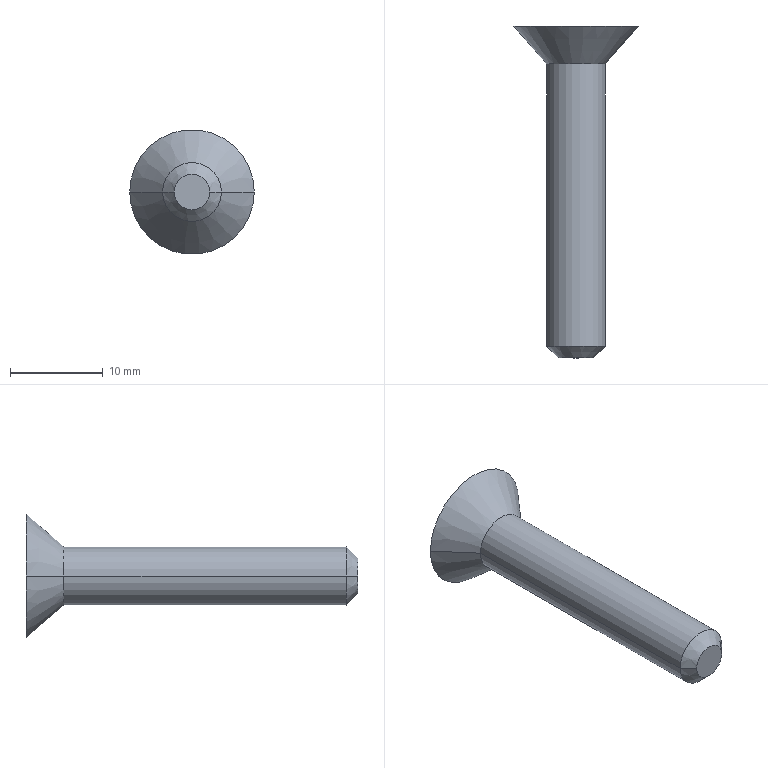Part | NX | features BREP 1 | 1 solid | 15 faces | box 13.46 x 35.839 x 13.46 mm | volume 1303 mm3 | plane 9 | cone 4 | cylinder 2 | commonest cylinder face diameters 6.35 x2
STEP:
#1=CARTESIAN_POINT('',(6.73,0.,0.));
#2=VERTEX_POINT('',#1);
#3=CARTESIAN_POINT('',(3.175,-4.089,0.));
#4=VERTEX_POINT('',#3);
#5=CARTESIAN_POINT('',(3.175,-4.089,0.));
#6=DIRECTION('',(0.6561,0.7547,0.));
#7=VECTOR('',#6,1000.);
#8=LINE('',#5,#7);
#9=EDGE_CURVE('',#2,#4,#8,.F.);
#10=ORIENTED_EDGE('',*,*,#9,.F.);
#11=CARTESIAN_POINT('',(-6.73,0.,0.));
#12=VERTEX_POINT('',#11);
#13=CARTESIAN_POINT('',(0.,0.,0.));
#14=DIRECTION('',(0.,-1.,0.));
#15=DIRECTION('',(1.,0.,0.));
#16=AXIS2_PLACEMENT_3D('',#13,#14,#15);
#17=CIRCLE('',#16,6.73);
#18=EDGE_CURVE('',#2,#12,#17,.T.);
#19=ORIENTED_EDGE('',*,*,#18,.T.);
#20=CARTESIAN_POINT('',(-3.175,-4.089,0.));
#21=VERTEX_POINT('',#20);
#22=CARTESIAN_POINT('',(-3.175,-4.089,0.));
#23=DIRECTION('',(-0.6561,0.7547,0.));
#24=VECTOR('',#23,1000.);
#25=LINE('',#22,#24);
#26=EDGE_CURVE('',#12,#21,#25,.F.);
#27=ORIENTED_EDGE('',*,*,#26,.T.);
#28=CARTESIAN_POINT('',(0.,-4.089,0.));
#29=DIRECTION('',(0.,-1.,0.));
#30=DIRECTION('',(1.,0.,0.));
#31=AXIS2_PLACEMENT_3D('',#28,#29,#30);
#32=CIRCLE('',#31,3.175);
#33=EDGE_CURVE('',#4,#21,#32,.T.);
#34=ORIENTED_EDGE('',*,*,#33,.F.);
#35=EDGE_LOOP('',(#10,#19,#27,#34));
#36=FACE_BOUND('',#35,.T.);
#37=CARTESIAN_POINT('',(0.,-2.045,0.));
#38=DIRECTION('',(0.,1.,0.));
#39=DIRECTION('',(1.,0.,0.));
#40=AXIS2_PLACEMENT_3D('',#37,#38,#39);
#41=CONICAL_SURFACE('',#40,4.952,0.7156);
#42=ADVANCED_FACE('',(#36),#41,.T.);
#43=CARTESIAN_POINT('',(-3.175,-34.569,0.));
#44=VERTEX_POINT('',#43);
#45=CARTESIAN_POINT('',(-3.175,-4.089,0.));
#46=DIRECTION('',(0.,-1.,0.));
#47=VECTOR('',#46,1000.);
#48=LINE('',#45,#47);
#49=EDGE_CURVE('',#21,#44,#48,.T.);
#50=ORIENTED_EDGE('',*,*,#49,.T.);
#51=CARTESIAN_POINT('',(3.175,-34.569,0.));
#52=VERTEX_POINT('',#51);
#53=CARTESIAN_POINT('',(0.,-34.569,0.));
#54=DIRECTION('',(0.,-1.,0.));
#55=DIRECTION('',(1.,0.,0.));
#56=AXIS2_PLACEMENT_3D('',#53,#54,#55);
#57=CIRCLE('',#56,3.175);
#58=EDGE_CURVE('',#52,#44,#57,.T.);
#59=ORIENTED_EDGE('',*,*,#58,.F.);
#60=CARTESIAN_POINT('',(3.175,-4.089,0.));
#61=DIRECTION('',(0.,-1.,0.));
#62=VECTOR('',#61,1000.);
#63=LINE('',#60,#62);
#64=EDGE_CURVE('',#4,#52,#63,.T.);
#65=ORIENTED_EDGE('',*,*,#64,.F.);
#66=ORIENTED_EDGE('',*,*,#33,.T.);
#67=EDGE_LOOP('',(#50,#59,#65,#66));
#68=FACE_BOUND('',#67,.T.);
#69=CARTESIAN_POINT('',(0.,-4.089,0.));
#70=DIRECTION('',(0.,-1.,0.));
#71=DIRECTION('',(1.,0.,0.));
#72=AXIS2_PLACEMENT_3D('',#69,#70,#71);
#73=CYLINDRICAL_SURFACE('',#72,3.175);
#74=ADVANCED_FACE('',(#68),#73,.T.);
#75=ORIENTED_EDGE('',*,*,#64,.T.);
#76=CARTESIAN_POINT('',(0.,-34.569,0.));
#77=DIRECTION('',(0.,-1.,0.));
#78=DIRECTION('',(-1.,0.,0.));
#79=AXIS2_PLACEMENT_3D('',#76,#77,#78);
#80=CIRCLE('',#79,3.175);
#81=EDGE_CURVE('',#44,#52,#80,.T.);
#82=ORIENTED_EDGE('',*,*,#81,.F.);
#83=ORIENTED_EDGE('',*,*,#49,.F.);
#84=CARTESIAN_POINT('',(0.,-4.089,0.));
#85=DIRECTION('',(0.,-1.,0.));
#86=DIRECTION('',(-1.,0.,0.));
#87=AXIS2_PLACEMENT_3D('',#84,#85,#86);
#88=CIRCLE('',#87,3.175);
#89=EDGE_CURVE('',#21,#4,#88,.T.);
#90=ORIENTED_EDGE('',*,*,#89,.T.);
#91=EDGE_LOOP('',(#75,#82,#83,#90));
#92=FACE_BOUND('',#91,.T.);
#93=CARTESIAN_POINT('',(0.,-4.089,0.));
#94=DIRECTION('',(0.,-1.,0.));
#95=DIRECTION('',(1.,0.,0.));
#96=AXIS2_PLACEMENT_3D('',#93,#94,#95);
#97=CYLINDRICAL_SURFACE('',#96,3.175);
#98=ADVANCED_FACE('',(#92),#97,.T.);
#99=ORIENTED_EDGE('',*,*,#26,.F.);
#100=CARTESIAN_POINT('',(0.,0.,0.));
#101=DIRECTION('',(0.,1.,0.));
#102=DIRECTION('',(1.,0.,0.));
#103=AXIS2_PLACEMENT_3D('',#100,#101,#102);
#104=CIRCLE('',#103,6.73);
#105=EDGE_CURVE('',#2,#12,#104,.T.);
#106=ORIENTED_EDGE('',*,*,#105,.F.);
#107=ORIENTED_EDGE('',*,*,#9,.T.);
#108=ORIENTED_EDGE('',*,*,#89,.F.);
#109=EDGE_LOOP('',(#99,#106,#107,#108));
#110=FACE_BOUND('',#109,.T.);
#111=CARTESIAN_POINT('',(0.,-2.045,0.));
#112=DIRECTION('',(0.,1.,0.));
#113=DIRECTION('',(1.,0.,0.));
#114=AXIS2_PLACEMENT_3D('',#111,#112,#113);
#115=CONICAL_SURFACE('',#114,4.952,0.7156);
#116=ADVANCED_FACE('',(#110),#115,.T.);
#117=ORIENTED_EDGE('',*,*,#18,.F.);
#118=ORIENTED_EDGE('',*,*,#105,.T.);
#119=EDGE_LOOP('',(#117,#118));
#120=FACE_BOUND('',#119,.T.);
#121=CARTESIAN_POINT('',(-1.984,0.,-1.146));
#122=VERTEX_POINT('',#121);
#123=CARTESIAN_POINT('',(-1.984,0.,1.146));
#124=VERTEX_POINT('',#123);
#125=CARTESIAN_POINT('',(-1.984,0.,-1.146));
#126=DIRECTION('',(0.,0.,1.));
#127=VECTOR('',#126,1000.);
#128=LINE('',#125,#127);
#129=EDGE_CURVE('',#122,#124,#128,.T.);
#130=ORIENTED_EDGE('',*,*,#129,.F.);
#131=CARTESIAN_POINT('',(0.,0.,-2.291));
#132=VERTEX_POINT('',#131);
#133=CARTESIAN_POINT('',(0.,0.,-2.291));
#134=DIRECTION('',(-0.866,0.,0.5));
#135=VECTOR('',#134,1000.);
#136=LINE('',#133,#135);
#137=EDGE_CURVE('',#132,#122,#136,.T.);
#138=ORIENTED_EDGE('',*,*,#137,.F.);
#139=CARTESIAN_POINT('',(1.984,0.,-1.146));
#140=VERTEX_POINT('',#139);
#141=CARTESIAN_POINT('',(1.984,0.,-1.146));
#142=DIRECTION('',(-0.866,0.,-0.5));
#143=VECTOR('',#142,1000.);
#144=LINE('',#141,#143);
#145=EDGE_CURVE('',#140,#132,#144,.T.);
#146=ORIENTED_EDGE('',*,*,#145,.F.);
#147=CARTESIAN_POINT('',(1.984,0.,1.146));
#148=VERTEX_POINT('',#147);
#149=CARTESIAN_POINT('',(1.984,0.,1.146));
#150=DIRECTION('',(0.,0.,-1.));
#151=VECTOR('',#150,1000.);
#152=LINE('',#149,#151);
#153=EDGE_CURVE('',#148,#140,#152,.T.);
#154=ORIENTED_EDGE('',*,*,#153,.F.);
#155=CARTESIAN_POINT('',(0.,0.,2.291));
#156=VERTEX_POINT('',#155);
#157=CARTESIAN_POINT('',(0.,0.,2.291));
#158=DIRECTION('',(0.866,0.,-0.5));
#159=VECTOR('',#158,1000.);
#160=LINE('',#157,#159);
#161=EDGE_CURVE('',#156,#148,#160,.T.);
#162=ORIENTED_EDGE('',*,*,#161,.F.);
#163=CARTESIAN_POINT('',(-1.984,0.,1.146));
#164=DIRECTION('',(0.866,0.,0.5));
#165=VECTOR('',#164,1000.);
#166=LINE('',#163,#165);
#167=EDGE_CURVE('',#124,#156,#166,.T.);
#168=ORIENTED_EDGE('',*,*,#167,.F.);
#169=EDGE_LOOP('',(#130,#138,#146,#154,#162,#168));
#170=FACE_BOUND('',#169,.T.);
#171=CARTESIAN_POINT('',(0.,0.,0.));
#172=DIRECTION('',(0.,-1.,0.));
#173=DIRECTION('',(0.,0.,-1.));
#174=AXIS2_PLACEMENT_3D('',#171,#172,#173);
#175=PLANE('',#174);
#176=ADVANCED_FACE('',(#120,#170),#175,.F.);
#177=CARTESIAN_POINT('',(0.,-1.27,2.291));
#178=VERTEX_POINT('',#177);
#179=CARTESIAN_POINT('',(0.,0.,2.291));
#180=DIRECTION('',(0.,-1.,0.));
#181=VECTOR('',#180,1000.);
#182=LINE('',#179,#181);
#183=EDGE_CURVE('',#156,#178,#182,.T.);
#184=ORIENTED_EDGE('',*,*,#183,.T.);
#185=CARTESIAN_POINT('',(-1.984,-1.27,1.146));
#186=VERTEX_POINT('',#185);
#187=CARTESIAN_POINT('',(-1.984,-1.27,1.146));
#188=DIRECTION('',(0.866,0.,0.5));
#189=VECTOR('',#188,1000.);
#190=LINE('',#187,#189);
#191=EDGE_CURVE('',#186,#178,#190,.T.);
#192=ORIENTED_EDGE('',*,*,#191,.F.);
#193=CARTESIAN_POINT('',(-1.984,0.,1.146));
#194=DIRECTION('',(0.,-1.,0.));
#195=VECTOR('',#194,1000.);
#196=LINE('',#193,#195);
#197=EDGE_CURVE('',#124,#186,#196,.T.);
#198=ORIENTED_EDGE('',*,*,#197,.F.);
#199=ORIENTED_EDGE('',*,*,#167,.T.);
#200=EDGE_LOOP('',(#184,#192,#198,#199));
#201=FACE_BOUND('',#200,.T.);
#202=CARTESIAN_POINT('',(-1.984,0.,1.146));
#203=DIRECTION('',(-0.5,0.,0.866));
#204=DIRECTION('',(0.,1.,0.));
#205=AXIS2_PLACEMENT_3D('',#202,#203,#204);
#206=PLANE('',#205);
#207=ADVANCED_FACE('',(#201),#206,.F.);
#208=ORIENTED_EDGE('',*,*,#197,.T.);
#209=CARTESIAN_POINT('',(-1.984,-1.27,-1.146));
#210=VERTEX_POINT('',#209);
#211=CARTESIAN_POINT('',(-1.984,-1.27,-1.146));
#212=DIRECTION('',(0.,0.,1.));
#213=VECTOR('',#212,1000.);
#214=LINE('',#211,#213);
#215=EDGE_CURVE('',#210,#186,#214,.T.);
#216=ORIENTED_EDGE('',*,*,#215,.F.);
#217=CARTESIAN_POINT('',(-1.984,0.,-1.146));
#218=DIRECTION('',(0.,-1.,0.));
#219=VECTOR('',#218,1000.);
#220=LINE('',#217,#219);
#221=EDGE_CURVE('',#122,#210,#220,.T.);
#222=ORIENTED_EDGE('',*,*,#221,.F.);
#223=ORIENTED_EDGE('',*,*,#129,.T.);
#224=EDGE_LOOP('',(#208,#216,#222,#223));
#225=FACE_BOUND('',#224,.T.);
#226=CARTESIAN_POINT('',(-1.984,0.,-1.146));
#227=DIRECTION('',(-1.,0.,0.));
#228=DIRECTION('',(0.,0.,1.));
#229=AXIS2_PLACEMENT_3D('',#226,#227,#228);
#230=PLANE('',#229);
#231=ADVANCED_FACE('',(#225),#230,.F.);
#232=ORIENTED_EDGE('',*,*,#221,.T.);
#233=CARTESIAN_POINT('',(0.,-1.27,-2.291));
#234=VERTEX_POINT('',#233);
#235=CARTESIAN_POINT('',(0.,-1.27,-2.291));
#236=DIRECTION('',(-0.866,0.,0.5));
#237=VECTOR('',#236,1000.);
#238=LINE('',#235,#237);
#239=EDGE_CURVE('',#234,#210,#238,.T.);
#240=ORIENTED_EDGE('',*,*,#239,.F.);
#241=CARTESIAN_POINT('',(0.,0.,-2.291));
#242=DIRECTION('',(0.,-1.,0.));
#243=VECTOR('',#242,1000.);
#244=LINE('',#241,#243);
#245=EDGE_CURVE('',#132,#234,#244,.T.);
#246=ORIENTED_EDGE('',*,*,#245,.F.);
#247=ORIENTED_EDGE('',*,*,#137,.T.);
#248=EDGE_LOOP('',(#232,#240,#246,#247));
#249=FACE_BOUND('',#248,.T.);
#250=CARTESIAN_POINT('',(0.,0.,-2.291));
#251=DIRECTION('',(-0.5,0.,-0.866));
#252=DIRECTION('',(-0.866,0.,0.5));
#253=AXIS2_PLACEMENT_3D('',#250,#251,#252);
#254=PLANE('',#253);
#255=ADVANCED_FACE('',(#249),#254,.F.);
#256=ORIENTED_EDGE('',*,*,#245,.T.);
#257=CARTESIAN_POINT('',(1.984,-1.27,-1.146));
#258=VERTEX_POINT('',#257);
#259=CARTESIAN_POINT('',(1.984,-1.27,-1.146));
#260=DIRECTION('',(-0.866,0.,-0.5));
#261=VECTOR('',#260,1000.);
#262=LINE('',#259,#261);
#263=EDGE_CURVE('',#258,#234,#262,.T.);
#264=ORIENTED_EDGE('',*,*,#263,.F.);
#265=CARTESIAN_POINT('',(1.984,0.,-1.146));
#266=DIRECTION('',(0.,-1.,0.));
#267=VECTOR('',#266,1000.);
#268=LINE('',#265,#267);
#269=EDGE_CURVE('',#140,#258,#268,.T.);
#270=ORIENTED_EDGE('',*,*,#269,.F.);
#271=ORIENTED_EDGE('',*,*,#145,.T.);
#272=EDGE_LOOP('',(#256,#264,#270,#271));
#273=FACE_BOUND('',#272,.T.);
#274=CARTESIAN_POINT('',(1.984,0.,-1.146));
#275=DIRECTION('',(0.5,0.,-0.866));
#276=DIRECTION('',(0.,-1.,0.));
#277=AXIS2_PLACEMENT_3D('',#274,#275,#276);
#278=PLANE('',#277);
#279=ADVANCED_FACE('',(#273),#278,.F.);
#280=ORIENTED_EDGE('',*,*,#269,.T.);
#281=CARTESIAN_POINT('',(1.984,-1.27,1.146));
#282=VERTEX_POINT('',#281);
#283=CARTESIAN_POINT('',(1.984,-1.27,1.146));
#284=DIRECTION('',(0.,0.,-1.));
#285=VECTOR('',#284,1000.);
#286=LINE('',#283,#285);
#287=EDGE_CURVE('',#282,#258,#286,.T.);
#288=ORIENTED_EDGE('',*,*,#287,.F.);
#289=CARTESIAN_POINT('',(1.984,0.,1.146));
#290=DIRECTION('',(0.,-1.,0.));
#291=VECTOR('',#290,1000.);
#292=LINE('',#289,#291);
#293=EDGE_CURVE('',#148,#282,#292,.T.);
#294=ORIENTED_EDGE('',*,*,#293,.F.);
#295=ORIENTED_EDGE('',*,*,#153,.T.);
#296=EDGE_LOOP('',(#280,#288,#294,#295));
#297=FACE_BOUND('',#296,.T.);
#298=CARTESIAN_POINT('',(1.984,0.,1.146));
#299=DIRECTION('',(1.,0.,0.));
#300=DIRECTION('',(0.,1.,0.));
#301=AXIS2_PLACEMENT_3D('',#298,#299,#300);
#302=PLANE('',#301);
#303=ADVANCED_FACE('',(#297),#302,.F.);
#304=ORIENTED_EDGE('',*,*,#293,.T.);
#305=CARTESIAN_POINT('',(0.,-1.27,2.291));
#306=DIRECTION('',(0.866,0.,-0.5));
#307=VECTOR('',#306,1000.);
#308=LINE('',#305,#307);
#309=EDGE_CURVE('',#178,#282,#308,.T.);
#310=ORIENTED_EDGE('',*,*,#309,.F.);
#311=ORIENTED_EDGE('',*,*,#183,.F.);
#312=ORIENTED_EDGE('',*,*,#161,.T.);
#313=EDGE_LOOP('',(#304,#310,#311,#312));
#314=FACE_BOUND('',#313,.T.);
#315=CARTESIAN_POINT('',(0.,0.,2.291));
#316=DIRECTION('',(0.5,0.,0.866));
#317=DIRECTION('',(0.,-1.,0.));
#318=AXIS2_PLACEMENT_3D('',#315,#316,#317);
#319=PLANE('',#318);
#320=ADVANCED_FACE('',(#314),#319,.F.);
#321=ORIENTED_EDGE('',*,*,#309,.T.);
#322=ORIENTED_EDGE('',*,*,#287,.T.);
#323=ORIENTED_EDGE('',*,*,#263,.T.);
#324=ORIENTED_EDGE('',*,*,#239,.T.);
#325=ORIENTED_EDGE('',*,*,#215,.T.);
#326=ORIENTED_EDGE('',*,*,#191,.T.);
#327=EDGE_LOOP('',(#321,#322,#323,#324,#325,#326));
#328=FACE_BOUND('',#327,.T.);
#329=CARTESIAN_POINT('',(0.,-1.27,0.));
#330=DIRECTION('',(0.,1.,0.));
#331=DIRECTION('',(1.,0.,0.));
#332=AXIS2_PLACEMENT_3D('',#329,#330,#331);
#333=PLANE('',#332);
#334=ADVANCED_FACE('',(#328),#333,.T.);
#335=CARTESIAN_POINT('',(-1.905,-35.839,0.));
#336=VERTEX_POINT('',#335);
#337=CARTESIAN_POINT('',(-1.905,-35.839,0.));
#338=DIRECTION('',(-0.7071,0.7071,0.));
#339=VECTOR('',#338,1000.);
#340=LINE('',#337,#339);
#341=EDGE_CURVE('',#336,#44,#340,.T.);
#342=ORIENTED_EDGE('',*,*,#341,.T.);
#343=ORIENTED_EDGE('',*,*,#81,.T.);
#344=CARTESIAN_POINT('',(1.905,-35.839,0.));
#345=VERTEX_POINT('',#344);
#346=CARTESIAN_POINT('',(1.905,-35.839,0.));
#347=DIRECTION('',(0.7071,0.7071,0.));
#348=VECTOR('',#347,1000.);
#349=LINE('',#346,#348);
#350=EDGE_CURVE('',#345,#52,#349,.T.);
#351=ORIENTED_EDGE('',*,*,#350,.F.);
#352=CARTESIAN_POINT('',(0.,-35.839,0.));
#353=DIRECTION('',(0.,-1.,0.));
#354=DIRECTION('',(-1.,0.,0.));
#355=AXIS2_PLACEMENT_3D('',#352,#353,#354);
#356=CIRCLE('',#355,1.905);
#357=EDGE_CURVE('',#336,#345,#356,.T.);
#358=ORIENTED_EDGE('',*,*,#357,.F.);
#359=EDGE_LOOP('',(#342,#343,#351,#358));
#360=FACE_BOUND('',#359,.T.);
#361=CARTESIAN_POINT('',(0.,-35.204,0.));
#362=DIRECTION('',(0.,1.,0.));
#363=DIRECTION('',(-1.,0.,0.));
#364=AXIS2_PLACEMENT_3D('',#361,#362,#363);
#365=CONICAL_SURFACE('',#364,2.54,0.7854);
#366=ADVANCED_FACE('',(#360),#365,.T.);
#367=ORIENTED_EDGE('',*,*,#357,.T.);
#368=CARTESIAN_POINT('',(0.,-35.839,0.));
#369=DIRECTION('',(0.,-1.,0.));
#370=DIRECTION('',(1.,0.,0.));
#371=AXIS2_PLACEMENT_3D('',#368,#369,#370);
#372=CIRCLE('',#371,1.905);
#373=EDGE_CURVE('',#345,#336,#372,.T.);
#374=ORIENTED_EDGE('',*,*,#373,.T.);
#375=EDGE_LOOP('',(#367,#374));
#376=FACE_BOUND('',#375,.T.);
#377=CARTESIAN_POINT('',(0.,-35.839,0.));
#378=DIRECTION('',(0.,-1.,0.));
#379=DIRECTION('',(0.,0.,-1.));
#380=AXIS2_PLACEMENT_3D('',#377,#378,#379);
#381=PLANE('',#380);
#382=ADVANCED_FACE('',(#376),#381,.T.);
#383=ORIENTED_EDGE('',*,*,#350,.T.);
#384=ORIENTED_EDGE('',*,*,#58,.T.);
#385=ORIENTED_EDGE('',*,*,#341,.F.);
#386=ORIENTED_EDGE('',*,*,#373,.F.);
#387=EDGE_LOOP('',(#383,#384,#385,#386));
#388=FACE_BOUND('',#387,.T.);
#389=CARTESIAN_POINT('',(0.,-35.204,0.));
#390=DIRECTION('',(0.,1.,0.));
#391=DIRECTION('',(-1.,0.,0.));
#392=AXIS2_PLACEMENT_3D('',#389,#390,#391);
#393=CONICAL_SURFACE('',#392,2.54,0.7854);
#394=ADVANCED_FACE('',(#388),#393,.T.);
#395=CLOSED_SHELL('',(#42,#74,#98,#116,#176,#207,#231,#255,#279,#303,#320,#334,#366,#382,#394));
#396=MANIFOLD_SOLID_BREP('',#395);
#397=(LENGTH_UNIT()NAMED_UNIT(*)SI_UNIT(.MILLI.,.METRE.));
#398=UNCERTAINTY_MEASURE_WITH_UNIT(LENGTH_MEASURE(0.00001),#397,'','');
#399=(NAMED_UNIT(*)PLANE_ANGLE_UNIT()SI_UNIT($,.RADIAN.));
#400=(NAMED_UNIT(*)SI_UNIT($,.STERADIAN.)SOLID_ANGLE_UNIT());
#401=(GEOMETRIC_REPRESENTATION_CONTEXT(3)GLOBAL_UNCERTAINTY_ASSIGNED_CONTEXT((#398))GLOBAL_UNIT_ASSIGNED_CONTEXT((#397,#399,#400))REPRESENTATION_CONTEXT('',''));
#402=ADVANCED_BREP_SHAPE_REPRESENTATION('',(#396),#401);